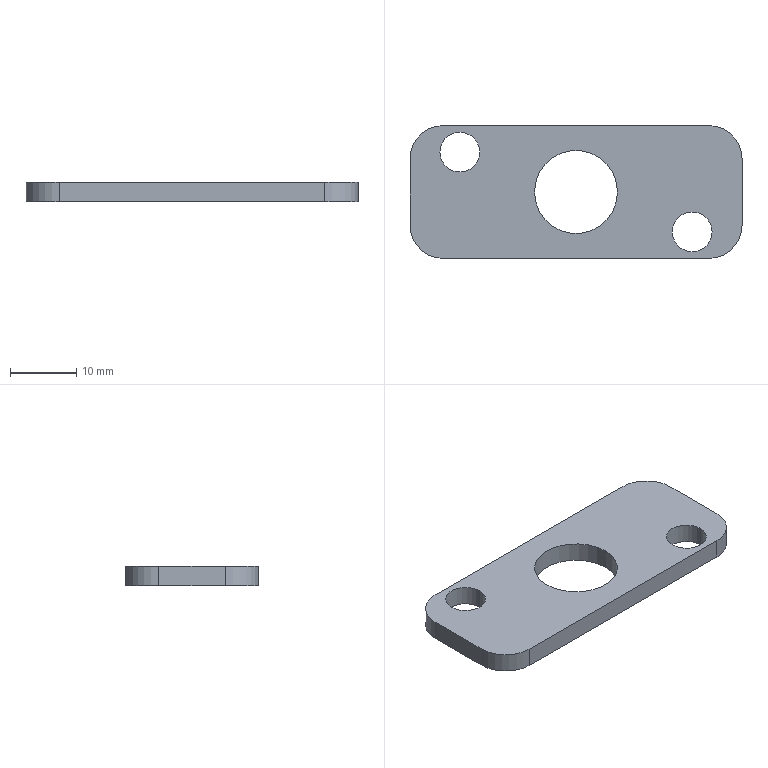Part | SolidWorks | features Extrusion 1 | 1 solid | 16 faces | box 50 x 20 x 3 mm | volume 2398 mm3 | cylinder 10 | plane 6 | commonest cylinder face diameters 6 x4 10 x4 12.5 x2
STEP:
#1=CARTESIAN_POINT('',(-6.25,0.,-1.5));
#2=VERTEX_POINT('',#1);
#3=CARTESIAN_POINT('',(6.25,0.,-1.5));
#4=VERTEX_POINT('',#3);
#5=CARTESIAN_POINT('',(0.,0.,-1.5));
#6=DIRECTION('',(0.,0.,1.));
#7=DIRECTION('',(-1.,0.,0.));
#8=AXIS2_PLACEMENT_3D('',#5,#6,#7);
#9=CIRCLE('',#8,6.25);
#10=EDGE_CURVE('',#2,#4,#9,.T.);
#11=ORIENTED_EDGE('',*,*,#10,.F.);
#12=CARTESIAN_POINT('',(-6.25,0.,1.5));
#13=VERTEX_POINT('',#12);
#14=CARTESIAN_POINT('',(-6.25,0.,-1.5));
#15=DIRECTION('',(0.,0.,1.));
#16=VECTOR('',#15,1000.);
#17=LINE('',#14,#16);
#18=EDGE_CURVE('',#2,#13,#17,.T.);
#19=ORIENTED_EDGE('',*,*,#18,.T.);
#20=CARTESIAN_POINT('',(6.25,0.,1.5));
#21=VERTEX_POINT('',#20);
#22=CARTESIAN_POINT('',(0.,0.,1.5));
#23=DIRECTION('',(0.,0.,1.));
#24=DIRECTION('',(-1.,0.,0.));
#25=AXIS2_PLACEMENT_3D('',#22,#23,#24);
#26=CIRCLE('',#25,6.25);
#27=EDGE_CURVE('',#13,#21,#26,.T.);
#28=ORIENTED_EDGE('',*,*,#27,.T.);
#29=CARTESIAN_POINT('',(6.25,0.,-1.5));
#30=DIRECTION('',(0.,0.,1.));
#31=VECTOR('',#30,1000.);
#32=LINE('',#29,#31);
#33=EDGE_CURVE('',#4,#21,#32,.T.);
#34=ORIENTED_EDGE('',*,*,#33,.F.);
#35=EDGE_LOOP('',(#11,#19,#28,#34));
#36=FACE_OUTER_BOUND('',#35,.T.);
#37=CARTESIAN_POINT('',(0.,0.,-1.5));
#38=DIRECTION('',(0.,0.,1.));
#39=DIRECTION('',(1.,0.,0.));
#40=AXIS2_PLACEMENT_3D('',#37,#38,#39);
#41=CYLINDRICAL_SURFACE('',#40,6.25);
#42=ADVANCED_FACE('',(#36),#41,.F.);
#43=CARTESIAN_POINT('',(14.5,-6.,-1.5));
#44=VERTEX_POINT('',#43);
#45=CARTESIAN_POINT('',(20.5,-6.,-1.5));
#46=VERTEX_POINT('',#45);
#47=CARTESIAN_POINT('',(17.5,-6.,-1.5));
#48=DIRECTION('',(0.,0.,1.));
#49=DIRECTION('',(-1.,0.,0.));
#50=AXIS2_PLACEMENT_3D('',#47,#48,#49);
#51=CIRCLE('',#50,3.);
#52=EDGE_CURVE('',#44,#46,#51,.T.);
#53=ORIENTED_EDGE('',*,*,#52,.F.);
#54=CARTESIAN_POINT('',(14.5,-6.,1.5));
#55=VERTEX_POINT('',#54);
#56=CARTESIAN_POINT('',(14.5,-6.,-1.5));
#57=DIRECTION('',(0.,0.,1.));
#58=VECTOR('',#57,1000.);
#59=LINE('',#56,#58);
#60=EDGE_CURVE('',#44,#55,#59,.T.);
#61=ORIENTED_EDGE('',*,*,#60,.T.);
#62=CARTESIAN_POINT('',(20.5,-6.,1.5));
#63=VERTEX_POINT('',#62);
#64=CARTESIAN_POINT('',(17.5,-6.,1.5));
#65=DIRECTION('',(0.,0.,1.));
#66=DIRECTION('',(-1.,0.,0.));
#67=AXIS2_PLACEMENT_3D('',#64,#65,#66);
#68=CIRCLE('',#67,3.);
#69=EDGE_CURVE('',#55,#63,#68,.T.);
#70=ORIENTED_EDGE('',*,*,#69,.T.);
#71=CARTESIAN_POINT('',(20.5,-6.,-1.5));
#72=DIRECTION('',(0.,0.,1.));
#73=VECTOR('',#72,1000.);
#74=LINE('',#71,#73);
#75=EDGE_CURVE('',#46,#63,#74,.T.);
#76=ORIENTED_EDGE('',*,*,#75,.F.);
#77=EDGE_LOOP('',(#53,#61,#70,#76));
#78=FACE_OUTER_BOUND('',#77,.T.);
#79=CARTESIAN_POINT('',(17.5,-6.,-1.5));
#80=DIRECTION('',(0.,0.,1.));
#81=DIRECTION('',(1.,0.,0.));
#82=AXIS2_PLACEMENT_3D('',#79,#80,#81);
#83=CYLINDRICAL_SURFACE('',#82,3.);
#84=ADVANCED_FACE('',(#78),#83,.F.);
#85=CARTESIAN_POINT('',(-20.5,6.,-1.5));
#86=VERTEX_POINT('',#85);
#87=CARTESIAN_POINT('',(-14.5,6.,-1.5));
#88=VERTEX_POINT('',#87);
#89=CARTESIAN_POINT('',(-17.5,6.,-1.5));
#90=DIRECTION('',(0.,0.,1.));
#91=DIRECTION('',(-1.,0.,0.));
#92=AXIS2_PLACEMENT_3D('',#89,#90,#91);
#93=CIRCLE('',#92,3.);
#94=EDGE_CURVE('',#86,#88,#93,.T.);
#95=ORIENTED_EDGE('',*,*,#94,.F.);
#96=CARTESIAN_POINT('',(-20.5,6.,1.5));
#97=VERTEX_POINT('',#96);
#98=CARTESIAN_POINT('',(-20.5,6.,-1.5));
#99=DIRECTION('',(0.,0.,1.));
#100=VECTOR('',#99,1000.);
#101=LINE('',#98,#100);
#102=EDGE_CURVE('',#86,#97,#101,.T.);
#103=ORIENTED_EDGE('',*,*,#102,.T.);
#104=CARTESIAN_POINT('',(-14.5,6.,1.5));
#105=VERTEX_POINT('',#104);
#106=CARTESIAN_POINT('',(-17.5,6.,1.5));
#107=DIRECTION('',(0.,0.,1.));
#108=DIRECTION('',(-1.,0.,0.));
#109=AXIS2_PLACEMENT_3D('',#106,#107,#108);
#110=CIRCLE('',#109,3.);
#111=EDGE_CURVE('',#97,#105,#110,.T.);
#112=ORIENTED_EDGE('',*,*,#111,.T.);
#113=CARTESIAN_POINT('',(-14.5,6.,-1.5));
#114=DIRECTION('',(0.,0.,1.));
#115=VECTOR('',#114,1000.);
#116=LINE('',#113,#115);
#117=EDGE_CURVE('',#88,#105,#116,.T.);
#118=ORIENTED_EDGE('',*,*,#117,.F.);
#119=EDGE_LOOP('',(#95,#103,#112,#118));
#120=FACE_OUTER_BOUND('',#119,.T.);
#121=CARTESIAN_POINT('',(-17.5,6.,-1.5));
#122=DIRECTION('',(0.,0.,1.));
#123=DIRECTION('',(1.,0.,0.));
#124=AXIS2_PLACEMENT_3D('',#121,#122,#123);
#125=CYLINDRICAL_SURFACE('',#124,3.);
#126=ADVANCED_FACE('',(#120),#125,.F.);
#127=CARTESIAN_POINT('',(-25.,-5.,1.5));
#128=VERTEX_POINT('',#127);
#129=CARTESIAN_POINT('',(-20.,-10.,1.5));
#130=VERTEX_POINT('',#129);
#131=CARTESIAN_POINT('',(-20.,-5.,1.5));
#132=DIRECTION('',(0.,0.,1.));
#133=DIRECTION('',(1.,0.,0.));
#134=AXIS2_PLACEMENT_3D('',#131,#132,#133);
#135=CIRCLE('',#134,5.);
#136=EDGE_CURVE('',#128,#130,#135,.T.);
#137=ORIENTED_EDGE('',*,*,#136,.F.);
#138=CARTESIAN_POINT('',(-25.,-5.,-1.5));
#139=VERTEX_POINT('',#138);
#140=CARTESIAN_POINT('',(-25.,-5.,-1.5));
#141=DIRECTION('',(0.,0.,1.));
#142=VECTOR('',#141,1000.);
#143=LINE('',#140,#142);
#144=EDGE_CURVE('',#139,#128,#143,.T.);
#145=ORIENTED_EDGE('',*,*,#144,.F.);
#146=CARTESIAN_POINT('',(-20.,-10.,-1.5));
#147=VERTEX_POINT('',#146);
#148=CARTESIAN_POINT('',(-20.,-5.,-1.5));
#149=DIRECTION('',(0.,0.,1.));
#150=DIRECTION('',(1.,0.,0.));
#151=AXIS2_PLACEMENT_3D('',#148,#149,#150);
#152=CIRCLE('',#151,5.);
#153=EDGE_CURVE('',#139,#147,#152,.T.);
#154=ORIENTED_EDGE('',*,*,#153,.T.);
#155=CARTESIAN_POINT('',(-20.,-10.,-1.5));
#156=DIRECTION('',(0.,0.,1.));
#157=VECTOR('',#156,1000.);
#158=LINE('',#155,#157);
#159=EDGE_CURVE('',#147,#130,#158,.T.);
#160=ORIENTED_EDGE('',*,*,#159,.T.);
#161=EDGE_LOOP('',(#137,#145,#154,#160));
#162=FACE_OUTER_BOUND('',#161,.T.);
#163=CARTESIAN_POINT('',(-20.,-5.,-1.5));
#164=DIRECTION('',(0.,0.,1.));
#165=DIRECTION('',(1.,0.,0.));
#166=AXIS2_PLACEMENT_3D('',#163,#164,#165);
#167=CYLINDRICAL_SURFACE('',#166,5.);
#168=ADVANCED_FACE('',(#162),#167,.T.);
#169=CARTESIAN_POINT('',(-25.,5.,1.5));
#170=VERTEX_POINT('',#169);
#171=CARTESIAN_POINT('',(-25.,5.,1.5));
#172=DIRECTION('',(0.,-1.,0.));
#173=VECTOR('',#172,1000.);
#174=LINE('',#171,#173);
#175=EDGE_CURVE('',#170,#128,#174,.T.);
#176=ORIENTED_EDGE('',*,*,#175,.F.);
#177=CARTESIAN_POINT('',(-25.,5.,-1.5));
#178=VERTEX_POINT('',#177);
#179=CARTESIAN_POINT('',(-25.,5.,-1.5));
#180=DIRECTION('',(0.,0.,1.));
#181=VECTOR('',#180,1000.);
#182=LINE('',#179,#181);
#183=EDGE_CURVE('',#178,#170,#182,.T.);
#184=ORIENTED_EDGE('',*,*,#183,.F.);
#185=CARTESIAN_POINT('',(-25.,5.,-1.5));
#186=DIRECTION('',(0.,-1.,0.));
#187=VECTOR('',#186,1000.);
#188=LINE('',#185,#187);
#189=EDGE_CURVE('',#178,#139,#188,.T.);
#190=ORIENTED_EDGE('',*,*,#189,.T.);
#191=ORIENTED_EDGE('',*,*,#144,.T.);
#192=EDGE_LOOP('',(#176,#184,#190,#191));
#193=FACE_OUTER_BOUND('',#192,.T.);
#194=CARTESIAN_POINT('',(-25.,5.,-1.5));
#195=DIRECTION('',(-1.,0.,0.));
#196=DIRECTION('',(0.,0.,1.));
#197=AXIS2_PLACEMENT_3D('',#194,#195,#196);
#198=PLANE('',#197);
#199=ADVANCED_FACE('',(#193),#198,.T.);
#200=CARTESIAN_POINT('',(-20.,10.,1.5));
#201=VERTEX_POINT('',#200);
#202=CARTESIAN_POINT('',(-20.,5.,1.5));
#203=DIRECTION('',(0.,0.,1.));
#204=DIRECTION('',(1.,0.,0.));
#205=AXIS2_PLACEMENT_3D('',#202,#203,#204);
#206=CIRCLE('',#205,5.);
#207=EDGE_CURVE('',#201,#170,#206,.T.);
#208=ORIENTED_EDGE('',*,*,#207,.F.);
#209=CARTESIAN_POINT('',(-20.,10.,-1.5));
#210=VERTEX_POINT('',#209);
#211=CARTESIAN_POINT('',(-20.,10.,-1.5));
#212=DIRECTION('',(0.,0.,1.));
#213=VECTOR('',#212,1000.);
#214=LINE('',#211,#213);
#215=EDGE_CURVE('',#210,#201,#214,.T.);
#216=ORIENTED_EDGE('',*,*,#215,.F.);
#217=CARTESIAN_POINT('',(-20.,5.,-1.5));
#218=DIRECTION('',(0.,0.,1.));
#219=DIRECTION('',(1.,0.,0.));
#220=AXIS2_PLACEMENT_3D('',#217,#218,#219);
#221=CIRCLE('',#220,5.);
#222=EDGE_CURVE('',#210,#178,#221,.T.);
#223=ORIENTED_EDGE('',*,*,#222,.T.);
#224=ORIENTED_EDGE('',*,*,#183,.T.);
#225=EDGE_LOOP('',(#208,#216,#223,#224));
#226=FACE_OUTER_BOUND('',#225,.T.);
#227=CARTESIAN_POINT('',(-20.,5.,-1.5));
#228=DIRECTION('',(0.,0.,1.));
#229=DIRECTION('',(1.,0.,0.));
#230=AXIS2_PLACEMENT_3D('',#227,#228,#229);
#231=CYLINDRICAL_SURFACE('',#230,5.);
#232=ADVANCED_FACE('',(#226),#231,.T.);
#233=CARTESIAN_POINT('',(20.,10.,1.5));
#234=VERTEX_POINT('',#233);
#235=CARTESIAN_POINT('',(20.,10.,1.5));
#236=DIRECTION('',(-1.,0.,0.));
#237=VECTOR('',#236,1000.);
#238=LINE('',#235,#237);
#239=EDGE_CURVE('',#234,#201,#238,.T.);
#240=ORIENTED_EDGE('',*,*,#239,.F.);
#241=CARTESIAN_POINT('',(20.,10.,-1.5));
#242=VERTEX_POINT('',#241);
#243=CARTESIAN_POINT('',(20.,10.,-1.5));
#244=DIRECTION('',(0.,0.,1.));
#245=VECTOR('',#244,1000.);
#246=LINE('',#243,#245);
#247=EDGE_CURVE('',#242,#234,#246,.T.);
#248=ORIENTED_EDGE('',*,*,#247,.F.);
#249=CARTESIAN_POINT('',(20.,10.,-1.5));
#250=DIRECTION('',(-1.,0.,0.));
#251=VECTOR('',#250,1000.);
#252=LINE('',#249,#251);
#253=EDGE_CURVE('',#242,#210,#252,.T.);
#254=ORIENTED_EDGE('',*,*,#253,.T.);
#255=ORIENTED_EDGE('',*,*,#215,.T.);
#256=EDGE_LOOP('',(#240,#248,#254,#255));
#257=FACE_OUTER_BOUND('',#256,.T.);
#258=CARTESIAN_POINT('',(20.,10.,-1.5));
#259=DIRECTION('',(0.,1.,0.));
#260=DIRECTION('',(0.,0.,1.));
#261=AXIS2_PLACEMENT_3D('',#258,#259,#260);
#262=PLANE('',#261);
#263=ADVANCED_FACE('',(#257),#262,.T.);
#264=CARTESIAN_POINT('',(25.,5.,1.5));
#265=VERTEX_POINT('',#264);
#266=CARTESIAN_POINT('',(20.,5.,1.5));
#267=DIRECTION('',(0.,0.,1.));
#268=DIRECTION('',(1.,0.,0.));
#269=AXIS2_PLACEMENT_3D('',#266,#267,#268);
#270=CIRCLE('',#269,5.);
#271=EDGE_CURVE('',#265,#234,#270,.T.);
#272=ORIENTED_EDGE('',*,*,#271,.F.);
#273=CARTESIAN_POINT('',(25.,5.,-1.5));
#274=VERTEX_POINT('',#273);
#275=CARTESIAN_POINT('',(25.,5.,-1.5));
#276=DIRECTION('',(0.,0.,1.));
#277=VECTOR('',#276,1000.);
#278=LINE('',#275,#277);
#279=EDGE_CURVE('',#274,#265,#278,.T.);
#280=ORIENTED_EDGE('',*,*,#279,.F.);
#281=CARTESIAN_POINT('',(20.,5.,-1.5));
#282=DIRECTION('',(0.,0.,1.));
#283=DIRECTION('',(1.,0.,0.));
#284=AXIS2_PLACEMENT_3D('',#281,#282,#283);
#285=CIRCLE('',#284,5.);
#286=EDGE_CURVE('',#274,#242,#285,.T.);
#287=ORIENTED_EDGE('',*,*,#286,.T.);
#288=ORIENTED_EDGE('',*,*,#247,.T.);
#289=EDGE_LOOP('',(#272,#280,#287,#288));
#290=FACE_OUTER_BOUND('',#289,.T.);
#291=CARTESIAN_POINT('',(20.,5.,-1.5));
#292=DIRECTION('',(0.,0.,1.));
#293=DIRECTION('',(1.,0.,0.));
#294=AXIS2_PLACEMENT_3D('',#291,#292,#293);
#295=CYLINDRICAL_SURFACE('',#294,5.);
#296=ADVANCED_FACE('',(#290),#295,.T.);
#297=CARTESIAN_POINT('',(25.,-5.,1.5));
#298=VERTEX_POINT('',#297);
#299=CARTESIAN_POINT('',(25.,-5.,1.5));
#300=DIRECTION('',(0.,1.,0.));
#301=VECTOR('',#300,1000.);
#302=LINE('',#299,#301);
#303=EDGE_CURVE('',#298,#265,#302,.T.);
#304=ORIENTED_EDGE('',*,*,#303,.F.);
#305=CARTESIAN_POINT('',(25.,-5.,-1.5));
#306=VERTEX_POINT('',#305);
#307=CARTESIAN_POINT('',(25.,-5.,-1.5));
#308=DIRECTION('',(0.,0.,1.));
#309=VECTOR('',#308,1000.);
#310=LINE('',#307,#309);
#311=EDGE_CURVE('',#306,#298,#310,.T.);
#312=ORIENTED_EDGE('',*,*,#311,.F.);
#313=CARTESIAN_POINT('',(25.,-5.,-1.5));
#314=DIRECTION('',(0.,1.,0.));
#315=VECTOR('',#314,1000.);
#316=LINE('',#313,#315);
#317=EDGE_CURVE('',#306,#274,#316,.T.);
#318=ORIENTED_EDGE('',*,*,#317,.T.);
#319=ORIENTED_EDGE('',*,*,#279,.T.);
#320=EDGE_LOOP('',(#304,#312,#318,#319));
#321=FACE_OUTER_BOUND('',#320,.T.);
#322=CARTESIAN_POINT('',(25.,-5.,-1.5));
#323=DIRECTION('',(1.,0.,0.));
#324=DIRECTION('',(0.,0.,-1.));
#325=AXIS2_PLACEMENT_3D('',#322,#323,#324);
#326=PLANE('',#325);
#327=ADVANCED_FACE('',(#321),#326,.T.);
#328=CARTESIAN_POINT('',(20.,-10.,1.5));
#329=VERTEX_POINT('',#328);
#330=CARTESIAN_POINT('',(20.,-5.,1.5));
#331=DIRECTION('',(0.,0.,1.));
#332=DIRECTION('',(1.,0.,0.));
#333=AXIS2_PLACEMENT_3D('',#330,#331,#332);
#334=CIRCLE('',#333,5.);
#335=EDGE_CURVE('',#329,#298,#334,.T.);
#336=ORIENTED_EDGE('',*,*,#335,.F.);
#337=CARTESIAN_POINT('',(20.,-10.,-1.5));
#338=VERTEX_POINT('',#337);
#339=CARTESIAN_POINT('',(20.,-10.,-1.5));
#340=DIRECTION('',(0.,0.,1.));
#341=VECTOR('',#340,1000.);
#342=LINE('',#339,#341);
#343=EDGE_CURVE('',#338,#329,#342,.T.);
#344=ORIENTED_EDGE('',*,*,#343,.F.);
#345=CARTESIAN_POINT('',(20.,-5.,-1.5));
#346=DIRECTION('',(0.,0.,1.));
#347=DIRECTION('',(1.,0.,0.));
#348=AXIS2_PLACEMENT_3D('',#345,#346,#347);
#349=CIRCLE('',#348,5.);
#350=EDGE_CURVE('',#338,#306,#349,.T.);
#351=ORIENTED_EDGE('',*,*,#350,.T.);
#352=ORIENTED_EDGE('',*,*,#311,.T.);
#353=EDGE_LOOP('',(#336,#344,#351,#352));
#354=FACE_OUTER_BOUND('',#353,.T.);
#355=CARTESIAN_POINT('',(20.,-5.,-1.5));
#356=DIRECTION('',(0.,0.,1.));
#357=DIRECTION('',(1.,0.,0.));
#358=AXIS2_PLACEMENT_3D('',#355,#356,#357);
#359=CYLINDRICAL_SURFACE('',#358,5.);
#360=ADVANCED_FACE('',(#354),#359,.T.);
#361=CARTESIAN_POINT('',(-20.,-10.,1.5));
#362=DIRECTION('',(1.,0.,0.));
#363=VECTOR('',#362,1000.);
#364=LINE('',#361,#363);
#365=EDGE_CURVE('',#130,#329,#364,.T.);
#366=ORIENTED_EDGE('',*,*,#365,.F.);
#367=ORIENTED_EDGE('',*,*,#159,.F.);
#368=CARTESIAN_POINT('',(-20.,-10.,-1.5));
#369=DIRECTION('',(1.,0.,0.));
#370=VECTOR('',#369,1000.);
#371=LINE('',#368,#370);
#372=EDGE_CURVE('',#147,#338,#371,.T.);
#373=ORIENTED_EDGE('',*,*,#372,.T.);
#374=ORIENTED_EDGE('',*,*,#343,.T.);
#375=EDGE_LOOP('',(#366,#367,#373,#374));
#376=FACE_OUTER_BOUND('',#375,.T.);
#377=CARTESIAN_POINT('',(-20.,-10.,-1.5));
#378=DIRECTION('',(0.,-1.,0.));
#379=DIRECTION('',(0.,0.,-1.));
#380=AXIS2_PLACEMENT_3D('',#377,#378,#379);
#381=PLANE('',#380);
#382=ADVANCED_FACE('',(#376),#381,.T.);
#383=CARTESIAN_POINT('',(0.,0.,-1.5));
#384=DIRECTION('',(0.,0.,1.));
#385=DIRECTION('',(-1.,0.,0.));
#386=AXIS2_PLACEMENT_3D('',#383,#384,#385);
#387=CIRCLE('',#386,6.25);
#388=EDGE_CURVE('',#4,#2,#387,.T.);
#389=ORIENTED_EDGE('',*,*,#388,.T.);
#390=ORIENTED_EDGE('',*,*,#10,.T.);
#391=EDGE_LOOP('',(#389,#390));
#392=FACE_BOUND('',#391,.T.);
#393=CARTESIAN_POINT('',(17.5,-6.,-1.5));
#394=DIRECTION('',(0.,0.,1.));
#395=DIRECTION('',(-1.,0.,0.));
#396=AXIS2_PLACEMENT_3D('',#393,#394,#395);
#397=CIRCLE('',#396,3.);
#398=EDGE_CURVE('',#46,#44,#397,.T.);
#399=ORIENTED_EDGE('',*,*,#398,.T.);
#400=ORIENTED_EDGE('',*,*,#52,.T.);
#401=EDGE_LOOP('',(#399,#400));
#402=FACE_BOUND('',#401,.T.);
#403=CARTESIAN_POINT('',(-17.5,6.,-1.5));
#404=DIRECTION('',(0.,0.,1.));
#405=DIRECTION('',(-1.,0.,0.));
#406=AXIS2_PLACEMENT_3D('',#403,#404,#405);
#407=CIRCLE('',#406,3.);
#408=EDGE_CURVE('',#88,#86,#407,.T.);
#409=ORIENTED_EDGE('',*,*,#408,.T.);
#410=ORIENTED_EDGE('',*,*,#94,.T.);
#411=EDGE_LOOP('',(#409,#410));
#412=FACE_BOUND('',#411,.T.);
#413=ORIENTED_EDGE('',*,*,#153,.F.);
#414=ORIENTED_EDGE('',*,*,#189,.F.);
#415=ORIENTED_EDGE('',*,*,#222,.F.);
#416=ORIENTED_EDGE('',*,*,#253,.F.);
#417=ORIENTED_EDGE('',*,*,#286,.F.);
#418=ORIENTED_EDGE('',*,*,#317,.F.);
#419=ORIENTED_EDGE('',*,*,#350,.F.);
#420=ORIENTED_EDGE('',*,*,#372,.F.);
#421=EDGE_LOOP('',(#413,#414,#415,#416,#417,#418,#419,#420));
#422=FACE_OUTER_BOUND('',#421,.T.);
#423=CARTESIAN_POINT('',(-20.,-5.,-1.5));
#424=DIRECTION('',(0.,0.,1.));
#425=DIRECTION('',(1.,0.,0.));
#426=AXIS2_PLACEMENT_3D('',#423,#424,#425);
#427=PLANE('',#426);
#428=ADVANCED_FACE('',(#392,#402,#412,#422),#427,.F.);
#429=CARTESIAN_POINT('',(0.,0.,1.5));
#430=DIRECTION('',(0.,0.,1.));
#431=DIRECTION('',(-1.,0.,0.));
#432=AXIS2_PLACEMENT_3D('',#429,#430,#431);
#433=CIRCLE('',#432,6.25);
#434=EDGE_CURVE('',#21,#13,#433,.T.);
#435=ORIENTED_EDGE('',*,*,#434,.F.);
#436=ORIENTED_EDGE('',*,*,#27,.F.);
#437=EDGE_LOOP('',(#435,#436));
#438=FACE_BOUND('',#437,.T.);
#439=CARTESIAN_POINT('',(17.5,-6.,1.5));
#440=DIRECTION('',(0.,0.,1.));
#441=DIRECTION('',(-1.,0.,0.));
#442=AXIS2_PLACEMENT_3D('',#439,#440,#441);
#443=CIRCLE('',#442,3.);
#444=EDGE_CURVE('',#63,#55,#443,.T.);
#445=ORIENTED_EDGE('',*,*,#444,.F.);
#446=ORIENTED_EDGE('',*,*,#69,.F.);
#447=EDGE_LOOP('',(#445,#446));
#448=FACE_BOUND('',#447,.T.);
#449=CARTESIAN_POINT('',(-17.5,6.,1.5));
#450=DIRECTION('',(0.,0.,1.));
#451=DIRECTION('',(-1.,0.,0.));
#452=AXIS2_PLACEMENT_3D('',#449,#450,#451);
#453=CIRCLE('',#452,3.);
#454=EDGE_CURVE('',#105,#97,#453,.T.);
#455=ORIENTED_EDGE('',*,*,#454,.F.);
#456=ORIENTED_EDGE('',*,*,#111,.F.);
#457=EDGE_LOOP('',(#455,#456));
#458=FACE_BOUND('',#457,.T.);
#459=ORIENTED_EDGE('',*,*,#136,.T.);
#460=ORIENTED_EDGE('',*,*,#365,.T.);
#461=ORIENTED_EDGE('',*,*,#335,.T.);
#462=ORIENTED_EDGE('',*,*,#303,.T.);
#463=ORIENTED_EDGE('',*,*,#271,.T.);
#464=ORIENTED_EDGE('',*,*,#239,.T.);
#465=ORIENTED_EDGE('',*,*,#207,.T.);
#466=ORIENTED_EDGE('',*,*,#175,.T.);
#467=EDGE_LOOP('',(#459,#460,#461,#462,#463,#464,#465,#466));
#468=FACE_OUTER_BOUND('',#467,.T.);
#469=CARTESIAN_POINT('',(-20.,-5.,1.5));
#470=DIRECTION('',(0.,0.,1.));
#471=DIRECTION('',(1.,0.,0.));
#472=AXIS2_PLACEMENT_3D('',#469,#470,#471);
#473=PLANE('',#472);
#474=ADVANCED_FACE('',(#438,#448,#458,#468),#473,.T.);
#475=ORIENTED_EDGE('',*,*,#102,.F.);
#476=ORIENTED_EDGE('',*,*,#408,.F.);
#477=ORIENTED_EDGE('',*,*,#117,.T.);
#478=ORIENTED_EDGE('',*,*,#454,.T.);
#479=EDGE_LOOP('',(#475,#476,#477,#478));
#480=FACE_OUTER_BOUND('',#479,.T.);
#481=CARTESIAN_POINT('',(-17.5,6.,-1.5));
#482=DIRECTION('',(0.,0.,1.));
#483=DIRECTION('',(1.,0.,0.));
#484=AXIS2_PLACEMENT_3D('',#481,#482,#483);
#485=CYLINDRICAL_SURFACE('',#484,3.);
#486=ADVANCED_FACE('',(#480),#485,.F.);
#487=ORIENTED_EDGE('',*,*,#60,.F.);
#488=ORIENTED_EDGE('',*,*,#398,.F.);
#489=ORIENTED_EDGE('',*,*,#75,.T.);
#490=ORIENTED_EDGE('',*,*,#444,.T.);
#491=EDGE_LOOP('',(#487,#488,#489,#490));
#492=FACE_OUTER_BOUND('',#491,.T.);
#493=CARTESIAN_POINT('',(17.5,-6.,-1.5));
#494=DIRECTION('',(0.,0.,1.));
#495=DIRECTION('',(1.,0.,0.));
#496=AXIS2_PLACEMENT_3D('',#493,#494,#495);
#497=CYLINDRICAL_SURFACE('',#496,3.);
#498=ADVANCED_FACE('',(#492),#497,.F.);
#499=ORIENTED_EDGE('',*,*,#18,.F.);
#500=ORIENTED_EDGE('',*,*,#388,.F.);
#501=ORIENTED_EDGE('',*,*,#33,.T.);
#502=ORIENTED_EDGE('',*,*,#434,.T.);
#503=EDGE_LOOP('',(#499,#500,#501,#502));
#504=FACE_OUTER_BOUND('',#503,.T.);
#505=CARTESIAN_POINT('',(0.,0.,-1.5));
#506=DIRECTION('',(0.,0.,1.));
#507=DIRECTION('',(1.,0.,0.));
#508=AXIS2_PLACEMENT_3D('',#505,#506,#507);
#509=CYLINDRICAL_SURFACE('',#508,6.25);
#510=ADVANCED_FACE('',(#504),#509,.F.);
#511=CLOSED_SHELL('',(#42,#84,#126,#168,#199,#232,#263,#296,#327,#360,#382,#428,#474,#486,#498,#510));
#512=MANIFOLD_SOLID_BREP('',#511);
#513=CARTESIAN_POINT('',(0.,0.,0.));
#514=DIRECTION('',(0.,0.,1.));
#515=DIRECTION('',(1.,0.,0.));
#516=AXIS2_PLACEMENT_3D('',#513,#514,#515);
#517=(LENGTH_UNIT()NAMED_UNIT(*)SI_UNIT(.MILLI.,.METRE.));
#518=UNCERTAINTY_MEASURE_WITH_UNIT(LENGTH_MEASURE(0.00001),#517,'','');
#519=(NAMED_UNIT(*)PLANE_ANGLE_UNIT()SI_UNIT($,.RADIAN.));
#520=(NAMED_UNIT(*)SI_UNIT($,.STERADIAN.)SOLID_ANGLE_UNIT());
#521=(GEOMETRIC_REPRESENTATION_CONTEXT(3)GLOBAL_UNCERTAINTY_ASSIGNED_CONTEXT((#518))GLOBAL_UNIT_ASSIGNED_CONTEXT((#517,#519,#520))REPRESENTATION_CONTEXT('',''));
#522=ADVANCED_BREP_SHAPE_REPRESENTATION('',(#512,#516),#521);